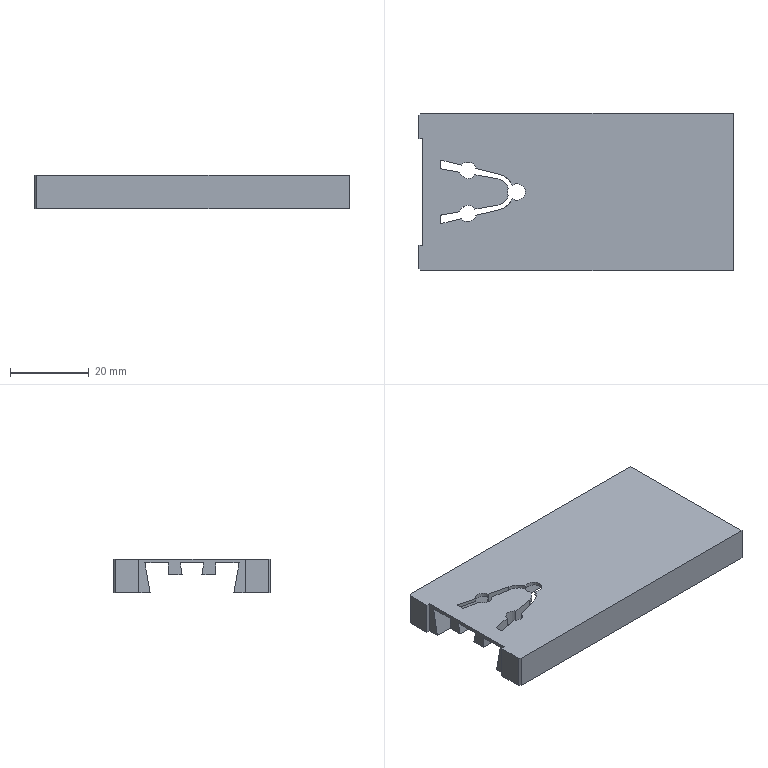Part | STEP file | slider | 1 solid | 64 faces | box 80 x 40 x 8.5 mm | volume 14605 mm3 | plane 41 | cylinder 19 | cone 4 | commonest cylinder face diameters 4.2 x6 0.6 x4 2.5 x4 6.8 x2 9.2 x2 3.5 x1